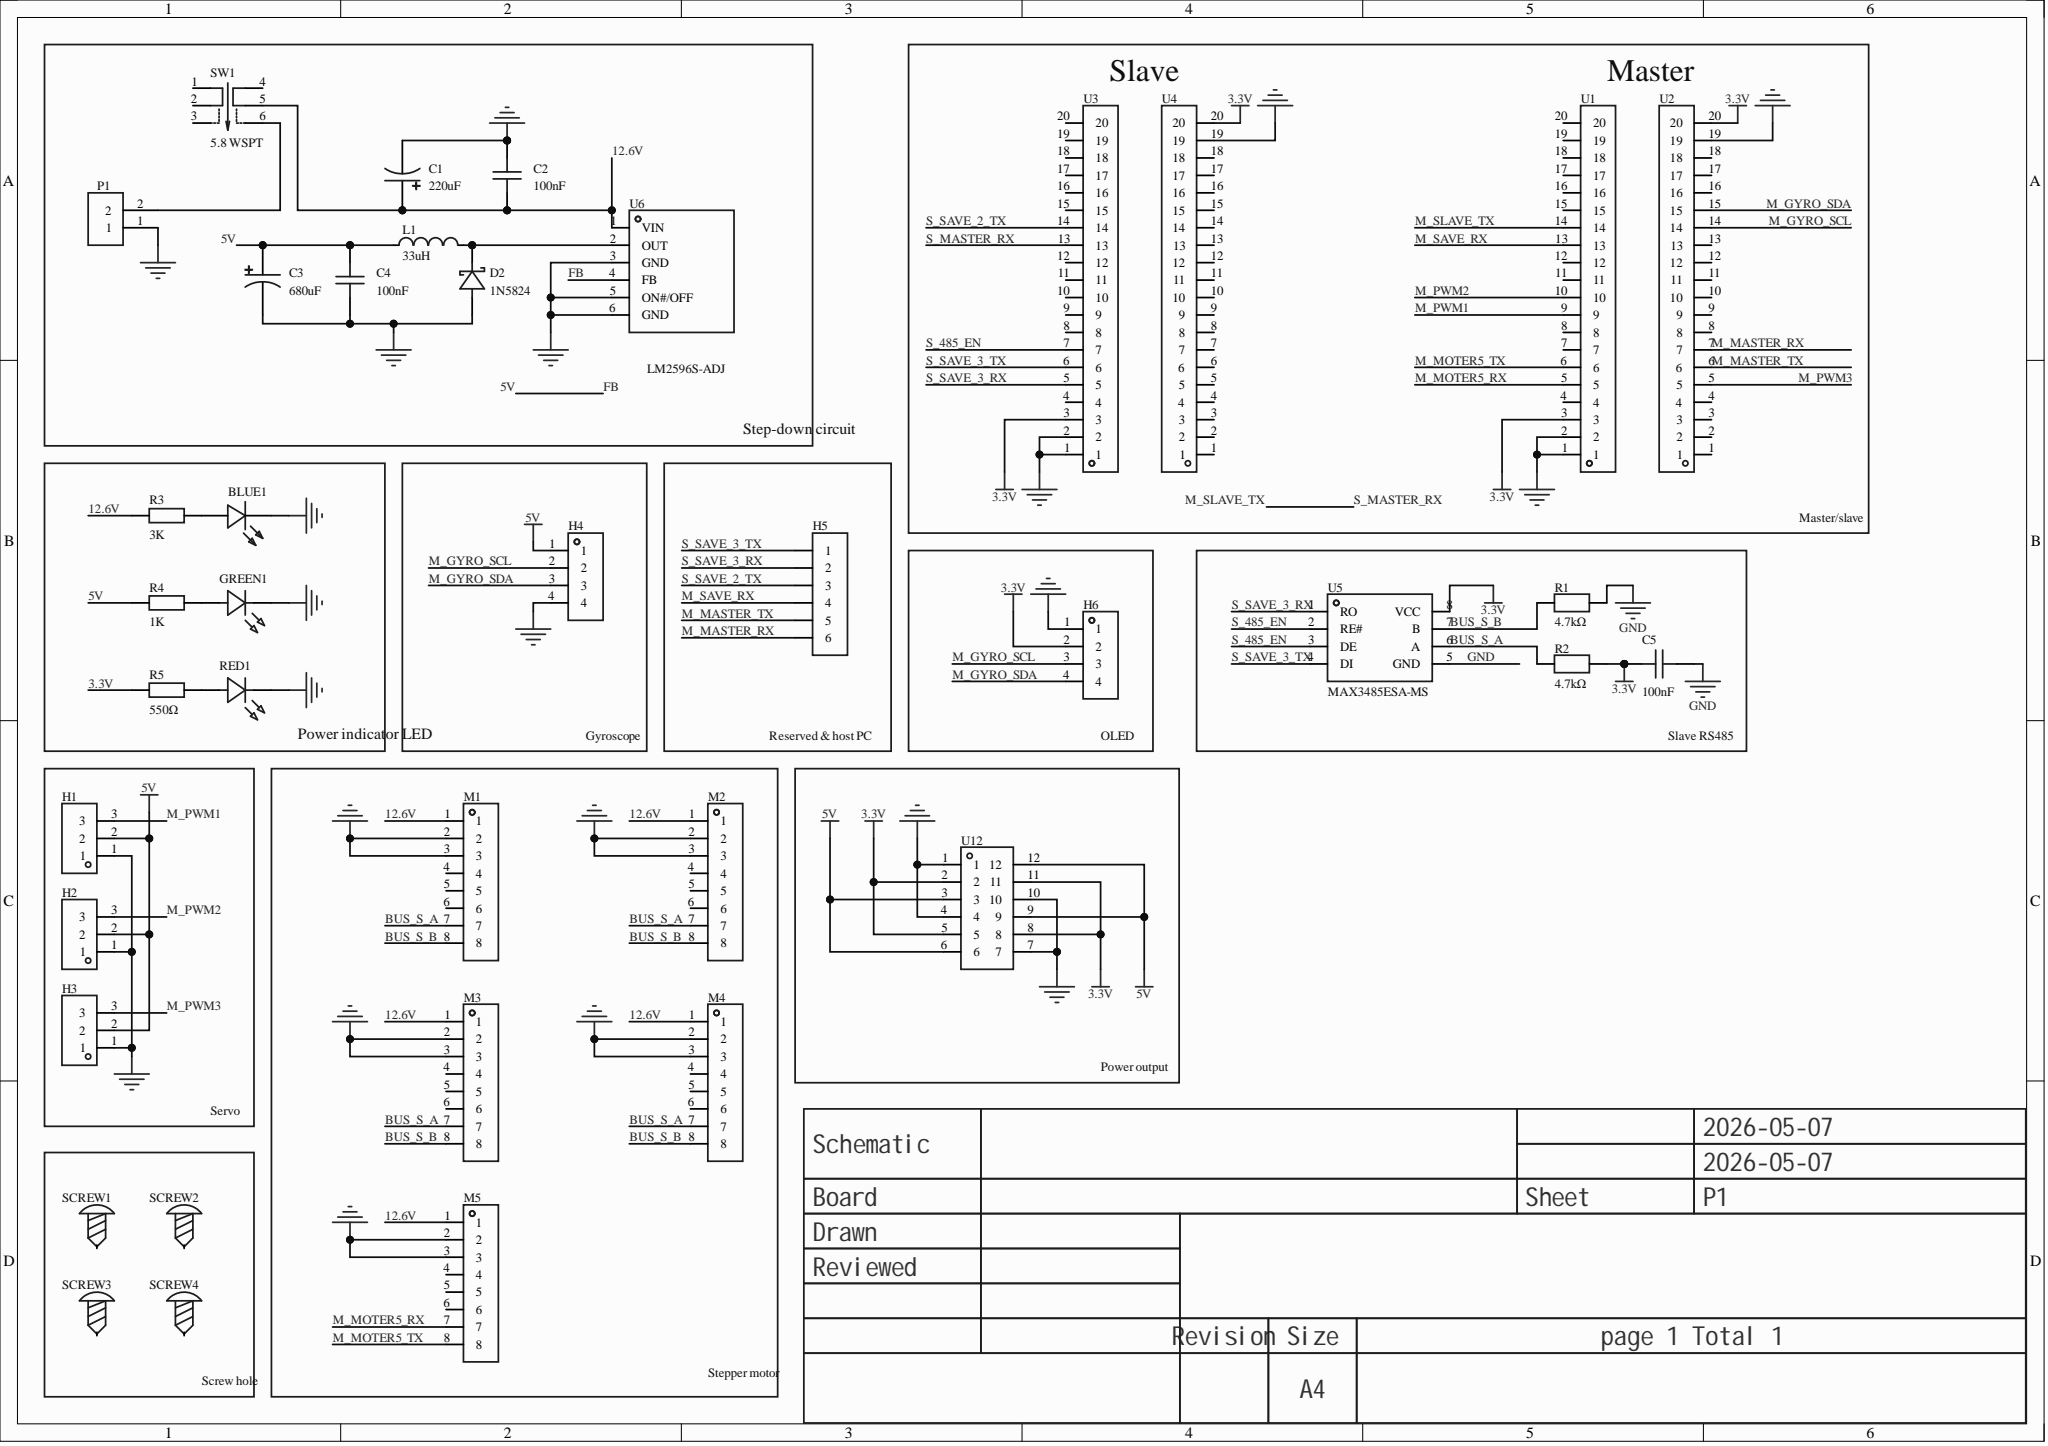Circuit board | Altium Designer | 39 parts | 26 nets
Bill of materials:
Comment,Description,Designator,Footprint,LibRef,Quantity
"SZYY0603B","Emitted color: Blue; Power: 100mW; Forward current: 5mA; Dominant wavelength: 460nm~475nm; Diode configuration: -; Lens color: Colorless transparent lens; Color temperature: -; Viewing angle: 120°; Packaging: -; Operating temperature: -40℃~+85℃;","BLUE1","LED0603-R-RD_BLUE","SZYY0603B","1"
"220uF","Capacitance: 220uF; Tolerance: ±20%; Rated voltage: 50V; Capacitor body diameter: 10mm; Capacitor body length: 10.2mm; Ripple current: -; Equivalent series resistance: -; Operating life: 2000hrs@105℃; Operating temperature: -45℃~+105℃;","C1","CAP-SMD_BD10.0-L10.3-W10.3-FD","EEEFK1H221P","1"
"100nF","","C2, C4","C0805","CAP_0805","2"
"680uF","Capacitance: 220uF; Tolerance: ±20%; Rated voltage: 35V; Capacitor body diameter: 8mm; Capacitor body length: 10.2mm; Ripple current: -; Equivalent series resistance: -; Operating life: 2000hrs@105℃; Operating temperature: -45℃~+105℃;","C3","CAP-SMD_BD8.0-L8.3-W8.3-FD","EEEFP1V221AP","1"
"100nF","Capacitance: 100nF; Tolerance: ±10%; Rated voltage: 50V; Temperature coefficient: X7R;","C5","C0603","CGA0603X7R104K500JT","1"
"1N5824","Diode configuration: Single; Forward voltage drop (Vf): 550mV@5A; DC reverse voltage (Vr): 30V; Rectified current: 5A;","D2","DO-27_BD5.3-L8.4-P12.40-D1.3-RD","1N5824_C7503125","1"
"XL-1608PGC-06","Lamp head type: -; Emitted color: Emerald green; Forward voltage (Vf): 2.6V~3V; Power: -; Forward current: -; Wavelength: 515nm~530nm; Diode configuration: -; Lens color: Green lens; Color temperature: -; Luminous intensity: 900mcd; Viewing angle: 120°; Packaging: SMD; Operating temperature: -;","GREEN1","LED0603-RD_GREEN","XL-1608PGC-06","1"
"PZ254V-11-03P","Pin structure: 1x3P; Pitch: 2.54mm; Row spacing: -; Round/square pin: Square pin; Mounting style: Through-hole; Rows: Single row; Total pins: 3P; Rated current: 3A; Rated voltage: 250V; Mating pin length: 6mm; Plastic height: 2.5mm; Tail length: 3mm; Operating temperature: -40℃~+105℃; Color: Black;","H1, H2, H3","HDR-TH_3P-P2.54-V-M","PZ254V-11-03P","3"
"PZ254V-11-04P","Pin structure: 1x4P; Pitch: 2.54mm; Row spacing: -; Round/square pin: Square pin; Mounting style: Through-hole; Rows: Single row; Total pins: 4P; Rated current: 3A; Rated voltage: 250V; Mating pin length: 6mm; Plastic height: 2.5mm; Tail length: 3mm; Contact material: -; Operating temperature: -40℃~+105℃;","H4, H6","HDR-TH_4P-P2.54-V-M","PZ254V-11-04P","2"
"2.54-1x6P straight pin","Pin structure: 1x6P; Pitch: 2.54mm; Row spacing: -; Round/square pin: Square pin; Mounting style: Through-hole; Rows: Single row; Total pins: 6P; Rated current: 3A; Rated voltage: -; Mating pin length: 6mm; Plastic height: 2.5mm; Tail length: 3mm; Contact material: Brass; Contact plating: Gold; Operating temperature: -40℃~+105℃; Color: Black;","H5","HDR-TH_6P-P2.54-V-M-1","2.54-1x6P直针","1"
"33uH","Type: -; Inductance: 33uH; Tolerance: ±20%; Rated current: 5.5A; Saturation current (Isat): 6A;","L1","IND-SMD_L13.45-W12.6","MWSA1206S-330MT","1"
"ZX-XH2.54-8PWZ","Pin structure: 1x8P; Pitch: 2.5mm; Mounting style: Right angle; Reference series: XH; Total pins: 8P; Rows: 1; Pins per row: 8; Row spacing: -; Rated current: 3A; Contact material: Brass; Contact plating: Tin; Operating temperature: -25℃~+85℃;","M1, M2, M3, M4, M5","CONN-TH_8P-P2.50_ZX-XH2.54-8PWZ","ZX-XH2.54-8PWZ","5"
"WJ500V-5.08-2P","Structure: 1x2P; Pitch: 5.08mm; Color: Green; Mounting style: Through-hole; Rated current: 18A; Rated voltage: 250V; Rows: 1; Wire gauge - AWG: 14~30; Wire gauge - mm²: 2.5; Pins per row: 2; Contact material: -; Contact plating: -; Operating temperature range: -40℃~+105℃; Soldering temperature (max): -;","P1","CONN-TH_2P-P5.00_WJ500V-5.08-2P","WJ500V-5.08-2P","1"
"4.7kΩ","Resistor type: Thick film resistor; Resistance: 10kΩ; Tolerance: ±1%; Power: 62.5mW; Operating voltage: 50V; Temperature coefficient: ±100ppm/?;","R1, R2","R0805","FRC0402F1002TS","2"
"3K","","R3","R0805","Res_0805","1"
"1K","","R4","R0805","Res_0805","1"
"550Ω","","R5","R0805","Res_0805","1"
"XL-1608SURC-06","Lamp head type: -; Emitted color: Red; Forward voltage (Vf): 2.3V; Power: 50mW; Forward current: 20mA; Wavelength: 620nm~630nm; Diode configuration: -; Lens color: Colorless transparent lens; Color temperature: -; Luminous intensity: 225mcd; Viewing angle: 120°; Packaging: SMD; Operating temperature: -40℃~+85℃;","RED1","LED0603-RD_RED","XL-1608SURC-06","1"
"","","SCREW1, SCREW2, SCREW3, SCREW4","M3螺丝","M3螺丝","4"
"5.8 WSPT","Circuit structure: DPDT; Self-lock/no-lock: No lock; Mounting style: Through-hole; Contact current: 100mA; Rated voltage: 30V; Lamp: No; Actuating force: 1.8N; Operating life: 5 thousand cycles;","SW1","SW-TH_6P-L5.8-W5.8-P2.00-LS4.5-TL_K8-5851E-L1","5.8 WSPT","1"
"ZX-PM2.54-1-20PY","Socket structure: 1x20P; Pitch: 2.54mm; Row spacing: -; Round/square hole: Square hole; Mounting type: Through-hole; Rows: Single row; Total holes: 20P; Rated current: -; Rated voltage: 1kV; Socket direction: Top; Plastic height: 8.5mm; Contact material: -; Contact plating: Gold; Operating temperature range: -40℃~+105℃;","U1, U2, U3, U4","HDR-TH_20P-P2.54-V-F","ZX-PM2.54-1-20PY","4"
"MAX3485ESA-MS","Type: Transceiver; Data rate: 12Mbps;","U5","SO-8_L4.9-W3.9-P1.27-LS5.9-BL","MAX3485ESA-MS","1"
"LM2596S-ADJ","","U6","TO-263-5_L10.2-W8.6-P1.70-LS14.4-BR","LM2596S-ADJ_C5276751","1"
"HX PZ2.54-3x4P ZZ","Pin structure: 3x4P; Pitch: 2.54mm; Row spacing: 2.54mm; Round/square pin: Square pin; Mounting style: Through-hole; Rows: Three rows; Total pins: 12P; Rated current: 3A; Rated voltage: 1kV; Mating pin length: 6mm; Plastic height: 2.5mm; Tail length: 3mm; Contact material: Brass; Contact plating: Gold; Operating temperature: -40℃~+105℃; Color: Black;","U12","HDR-TH_12P-P2.54-V-M-R3-C4-S2.54","HX PZ2.54-3x4P ZZ","1"
Netlist (Protel format):
[
BLUE1
LED0603-R-RD_BLUE
SZYY0603B



]
[
C1
CAP-SMD_BD10.0-L10.3-W10.3-FD
220uF



]
[
C2
C0805
100nF



]
[
C3
CAP-SMD_BD8.0-L8.3-W8.3-FD
680uF



]
[
C4
C0805
100nF



]
[
C5
C0603
100nF



]
[
D2
DO-27_BD5.3-L8.4-P12.40-D1.3-RD
1N5824



]
[
GREEN1
LED0603-RD_GREEN
XL-1608PGC-06



]
[
H1
HDR-TH_3P-P2.54-V-M
PZ254V-11-03P



]
[
H2
HDR-TH_3P-P2.54-V-M
PZ254V-11-03P



]
[
H3
HDR-TH_3P-P2.54-V-M
PZ254V-11-03P



]
[
H4
HDR-TH_4P-P2.54-V-M
PZ254V-11-04P



]
[
H5
HDR-TH_6P-P2.54-V-M-1
2.54-1x6P straight pin



]
[
H6
HDR-TH_4P-P2.54-V-M
PZ254V-11-04P



]
[
L1
IND-SMD_L13.45-W12.6
33uH



]
[
M1
CONN-TH_8P-P2.50_ZX-XH2.54-8PWZ
ZX-XH2.54-8PWZ



]
[
M2
CONN-TH_8P-P2.50_ZX-XH2.54-8PWZ
ZX-XH2.54-8PWZ



]
[
M3
CONN-TH_8P-P2.50_ZX-XH2.54-8PWZ
ZX-XH2.54-8PWZ



]
[
M4
CONN-TH_8P-P2.50_ZX-XH2.54-8PWZ
ZX-XH2.54-8PWZ



]
[
M5
CONN-TH_8P-P2.50_ZX-XH2.54-8PWZ
ZX-XH2.54-8PWZ



]
[
P1
CONN-TH_2P-P5.00_WJ500V-5.08-2P
WJ500V-5.08-2P



]
[
R1
R0805
4.7kΩ



]
[
R2
R0805
4.7kΩ



]
[
R3
R0805
3K



]
[
R4
R0805
1K



]
[
R5
R0805
550Ω



]
[
RED1
LED0603-RD_RED
XL-1608SURC-06



]
[
SCREW1
M3螺丝




]
[
SCREW2
M3螺丝




]
[
SCREW3
M3螺丝




]
[
SCREW4
M3螺丝




]
[
SW1
SW-TH_6P-L5.8-W5.8-P2.00-LS4.5-TL_K8-5851E-L1
5.8 WSPT



]
[
U1
HDR-TH_20P-P2.54-V-F
ZX-PM2.54-1-20PY



]
[
U2
HDR-TH_20P-P2.54-V-F
ZX-PM2.54-1-20PY



]
[
U3
HDR-TH_20P-P2.54-V-F
ZX-PM2.54-1-20PY



]
[
U4
HDR-TH_20P-P2.54-V-F
ZX-PM2.54-1-20PY



]
[
U5
SO-8_L4.9-W3.9-P1.27-LS5.9-BL
MAX3485ESA-MS



]
[
U6
TO-263-5_L10.2-W8.6-P1.70-LS14.4-BR
LM2596S-ADJ



]
[
U12
HDR-TH_12P-P2.54-V-M-R3-C4-S2.54
HX PZ2.54-3x4P ZZ



]
(
S_SAVE_3_TX
H5-1
U3-6
U5-4
)
(
S_SAVE_3_RX
H5-2
U3-5
U5-1
)
(
S_SAVE_2_TX
H5-3
U3-14
)
(
S_485_EN
U3-7
U5-2
U5-3
)
(
NetR5_1
R5-1
RED1-2
)
(
NetP1_2
P1-2
SW1-6
)
(
NetGREEN1_2
GREEN1-2
R4-1
)
(
NetD2_1
D2-1
L1-2
U6-2
)
(
NetBLUE1_1
BLUE1-1
R3-1
)
(
M_SLAVE_TX
U1-14
U3-13
)
(
M_SAVE_RX
H5-4
U1-13
)
(
M_PWM3
H3-3
U2-5
)
(
M_PWM2
H2-3
U1-10
)
(
M_PWM1
H1-3
U1-9
)
(
M_MOTER5_TX
M5-8
U1-6
)
(
M_MOTER5_RX
M5-7
U1-5
)
(
M_MASTER_TX
H5-5
U2-6
)
(
M_MASTER_RX
H5-6
U2-7
)
(
M_GYRO_SDA
H4-3
H6-4
U2-15
)
(
M_GYRO_SCL
H4-2
H6-3
U2-14
)
(
GND
BLUE1-2
C1-2
C2-1
C3-2
C4-1
C5-2
D2-2
GREEN1-1
H1-1
H2-1
H3-1
H4-4
H6-1
M1-2
M1-3
M2-2
M2-3
M3-2
M3-3
M4-2
M4-3
M5-2
M5-3
P1-1
R1-2
RED1-1
U1-1
U1-2
U2-19
U3-1
U3-2
U4-19
U5-5
U6-3
U6-5
U6-6
U12-1
U12-4
U12-7
U12-10
)
(
BUS_S_B
M1-8
M2-8
M3-8
M4-8
R1-1
U5-7
)
(
BUS_S_A
M1-7
M2-7
M3-7
M4-7
R2-1
U5-6
)
(
12.6V
C1-1
C2-2
M1-1
M2-1
M3-1
M4-1
M5-1
R3-2
SW1-5
U6-1
)
(
5V
C3-1
C4-2
H1-2
H2-2
H3-2
H4-1
L1-1
R4-2
U6-4
U12-3
U12-6
U12-9
U12-12
)
(
3.3V
C5-1
H6-2
R2-2
R5-2
U1-3
U2-20
U3-3
U4-20
U5-8
U12-2
U12-5
U12-8
U12-11
)